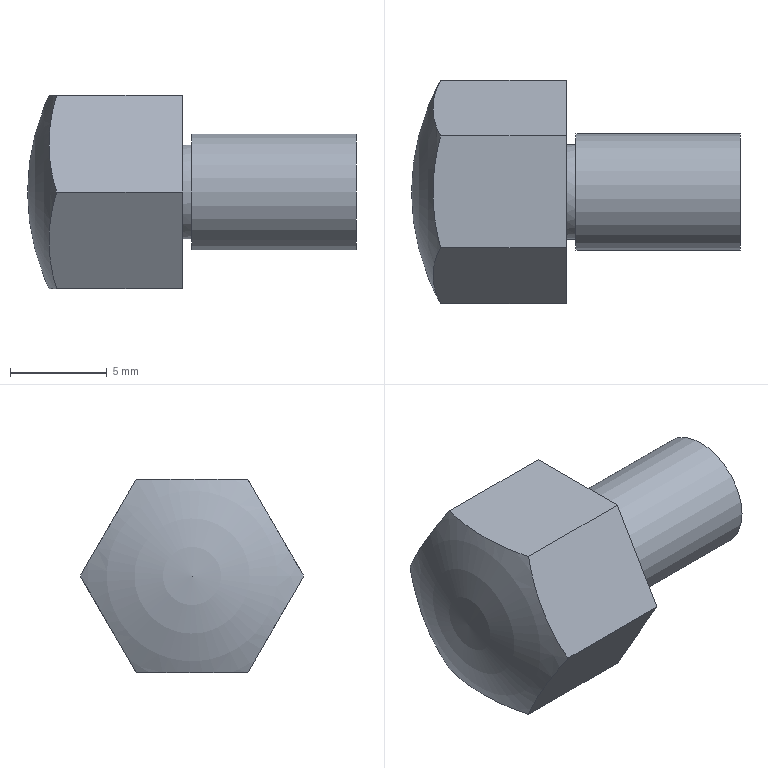Part | NX | features 5003_314_BSTEH10B 2 | 1 solid | 12 faces | box 17 x 11.547 x 10 mm | volume 889.716 mm3 | plane 9 | cylinder 2 | torus 1 | commonest cylinder face diameters 4.9 x1 6 x1
STEP:
#1=CARTESIAN_POINT('',(38.1,-177.774,-220.));
#2=VERTEX_POINT('',#1);
#3=CARTESIAN_POINT('',(38.1,-174.887,-215.));
#4=VERTEX_POINT('',#3);
#5=CARTESIAN_POINT('',(38.1,-177.774,-220.));
#6=CARTESIAN_POINT('',(37.578,-176.829,-218.364));
#7=CARTESIAN_POINT('',(37.578,-175.831,-216.636));
#8=CARTESIAN_POINT('',(38.1,-174.887,-215.));
#9=B_SPLINE_CURVE_WITH_KNOTS('',3,(#5,#6,#7,#8),.UNSPECIFIED.,.F.,.F.,(4,4),(0.000000237,0.00582),.UNSPECIFIED.);
#10=EDGE_CURVE('',#2,#4,#9,.T.);
#11=ORIENTED_EDGE('',*,*,#10,.F.);
#12=CARTESIAN_POINT('',(44.6,-177.774,-220.));
#13=VERTEX_POINT('',#12);
#14=CARTESIAN_POINT('',(36.6,-177.774,-220.));
#15=DIRECTION('',(1.,0.,0.));
#16=VECTOR('',#15,1000.);
#17=LINE('',#14,#16);
#18=EDGE_CURVE('',#2,#13,#17,.T.);
#19=ORIENTED_EDGE('',*,*,#18,.T.);
#20=CARTESIAN_POINT('',(44.6,-174.887,-215.));
#21=VERTEX_POINT('',#20);
#22=CARTESIAN_POINT('',(44.6,-174.887,-215.));
#23=DIRECTION('',(0.,-0.5,-0.866));
#24=VECTOR('',#23,1000.);
#25=LINE('',#22,#24);
#26=EDGE_CURVE('',#21,#13,#25,.T.);
#27=ORIENTED_EDGE('',*,*,#26,.F.);
#28=CARTESIAN_POINT('',(36.6,-174.887,-215.));
#29=DIRECTION('',(1.,0.,0.));
#30=VECTOR('',#29,1000.);
#31=LINE('',#28,#30);
#32=EDGE_CURVE('',#4,#21,#31,.T.);
#33=ORIENTED_EDGE('',*,*,#32,.F.);
#34=EDGE_LOOP('',(#11,#19,#27,#33));
#35=FACE_BOUND('',#34,.T.);
#36=CARTESIAN_POINT('',(36.6,-174.887,-215.));
#37=DIRECTION('',(0.,-0.866,0.5));
#38=DIRECTION('',(0.,-0.5,-0.866));
#39=AXIS2_PLACEMENT_3D('',#36,#37,#38);
#40=PLANE('',#39);
#41=ADVANCED_FACE('',(#35),#40,.T.);
#42=CARTESIAN_POINT('',(38.1,-169.113,-215.));
#43=VERTEX_POINT('',#42);
#44=CARTESIAN_POINT('',(38.1,-174.887,-215.));
#45=CARTESIAN_POINT('',(37.582,-173.011,-215.));
#46=CARTESIAN_POINT('',(37.582,-170.987,-215.));
#47=CARTESIAN_POINT('',(38.1,-169.113,-215.));
#48=B_SPLINE_CURVE_WITH_KNOTS('',3,(#44,#45,#46,#47),.UNSPECIFIED.,.F.,.F.,(4,4),(0.06513,0.07094),.UNSPECIFIED.);
#49=EDGE_CURVE('',#4,#43,#48,.T.);
#50=ORIENTED_EDGE('',*,*,#49,.F.);
#51=ORIENTED_EDGE('',*,*,#32,.T.);
#52=CARTESIAN_POINT('',(44.6,-169.113,-215.));
#53=VERTEX_POINT('',#52);
#54=CARTESIAN_POINT('',(44.6,-169.113,-215.));
#55=DIRECTION('',(0.,-1.,0.));
#56=VECTOR('',#55,1000.);
#57=LINE('',#54,#56);
#58=EDGE_CURVE('',#53,#21,#57,.T.);
#59=ORIENTED_EDGE('',*,*,#58,.F.);
#60=CARTESIAN_POINT('',(36.6,-169.113,-215.));
#61=DIRECTION('',(1.,0.,0.));
#62=VECTOR('',#61,1000.);
#63=LINE('',#60,#62);
#64=EDGE_CURVE('',#43,#53,#63,.T.);
#65=ORIENTED_EDGE('',*,*,#64,.F.);
#66=EDGE_LOOP('',(#50,#51,#59,#65));
#67=FACE_BOUND('',#66,.T.);
#68=CARTESIAN_POINT('',(36.6,-169.113,-215.));
#69=DIRECTION('',(0.,0.,1.));
#70=DIRECTION('',(-1.,0.,0.));
#71=AXIS2_PLACEMENT_3D('',#68,#69,#70);
#72=PLANE('',#71);
#73=ADVANCED_FACE('',(#67),#72,.T.);
#74=CARTESIAN_POINT('',(38.1,-166.226,-220.));
#75=VERTEX_POINT('',#74);
#76=CARTESIAN_POINT('',(38.1,-169.113,-215.));
#77=CARTESIAN_POINT('',(37.578,-168.169,-216.636));
#78=CARTESIAN_POINT('',(37.578,-167.171,-218.364));
#79=CARTESIAN_POINT('',(38.1,-166.226,-220.));
#80=B_SPLINE_CURVE_WITH_KNOTS('',3,(#76,#77,#78,#79),.UNSPECIFIED.,.F.,.F.,(4,4),(0.000000237,0.00582),.UNSPECIFIED.);
#81=EDGE_CURVE('',#43,#75,#80,.T.);
#82=ORIENTED_EDGE('',*,*,#81,.F.);
#83=ORIENTED_EDGE('',*,*,#64,.T.);
#84=CARTESIAN_POINT('',(44.6,-166.226,-220.));
#85=VERTEX_POINT('',#84);
#86=CARTESIAN_POINT('',(44.6,-166.226,-220.));
#87=DIRECTION('',(0.,-0.5,0.866));
#88=VECTOR('',#87,1000.);
#89=LINE('',#86,#88);
#90=EDGE_CURVE('',#85,#53,#89,.T.);
#91=ORIENTED_EDGE('',*,*,#90,.F.);
#92=CARTESIAN_POINT('',(36.6,-166.226,-220.));
#93=DIRECTION('',(1.,0.,0.));
#94=VECTOR('',#93,1000.);
#95=LINE('',#92,#94);
#96=EDGE_CURVE('',#75,#85,#95,.T.);
#97=ORIENTED_EDGE('',*,*,#96,.F.);
#98=EDGE_LOOP('',(#82,#83,#91,#97));
#99=FACE_BOUND('',#98,.T.);
#100=CARTESIAN_POINT('',(36.6,-166.226,-220.));
#101=DIRECTION('',(0.,0.866,0.5));
#102=DIRECTION('',(0.,-0.5,0.866));
#103=AXIS2_PLACEMENT_3D('',#100,#101,#102);
#104=PLANE('',#103);
#105=ADVANCED_FACE('',(#99),#104,.T.);
#106=CARTESIAN_POINT('',(38.1,-169.113,-225.));
#107=VERTEX_POINT('',#106);
#108=CARTESIAN_POINT('',(38.1,-166.226,-220.));
#109=CARTESIAN_POINT('',(37.578,-167.171,-221.636));
#110=CARTESIAN_POINT('',(37.578,-168.169,-223.364));
#111=CARTESIAN_POINT('',(38.1,-169.113,-225.));
#112=B_SPLINE_CURVE_WITH_KNOTS('',3,(#108,#109,#110,#111),.UNSPECIFIED.,.F.,.F.,(4,4),(0.000000237,0.00582),.UNSPECIFIED.);
#113=EDGE_CURVE('',#75,#107,#112,.T.);
#114=ORIENTED_EDGE('',*,*,#113,.F.);
#115=ORIENTED_EDGE('',*,*,#96,.T.);
#116=CARTESIAN_POINT('',(44.6,-169.113,-225.));
#117=VERTEX_POINT('',#116);
#118=CARTESIAN_POINT('',(44.6,-169.113,-225.));
#119=DIRECTION('',(0.,0.5,0.866));
#120=VECTOR('',#119,1000.);
#121=LINE('',#118,#120);
#122=EDGE_CURVE('',#117,#85,#121,.T.);
#123=ORIENTED_EDGE('',*,*,#122,.F.);
#124=CARTESIAN_POINT('',(36.6,-169.113,-225.));
#125=DIRECTION('',(1.,0.,0.));
#126=VECTOR('',#125,1000.);
#127=LINE('',#124,#126);
#128=EDGE_CURVE('',#107,#117,#127,.T.);
#129=ORIENTED_EDGE('',*,*,#128,.F.);
#130=EDGE_LOOP('',(#114,#115,#123,#129));
#131=FACE_BOUND('',#130,.T.);
#132=CARTESIAN_POINT('',(36.6,-169.113,-225.));
#133=DIRECTION('',(0.,0.866,-0.5));
#134=DIRECTION('',(0.,0.5,0.866));
#135=AXIS2_PLACEMENT_3D('',#132,#133,#134);
#136=PLANE('',#135);
#137=ADVANCED_FACE('',(#131),#136,.T.);
#138=CARTESIAN_POINT('',(38.1,-174.887,-225.));
#139=VERTEX_POINT('',#138);
#140=CARTESIAN_POINT('',(38.1,-169.113,-225.));
#141=CARTESIAN_POINT('',(37.582,-170.989,-225.));
#142=CARTESIAN_POINT('',(37.582,-173.013,-225.));
#143=CARTESIAN_POINT('',(38.1,-174.887,-225.));
#144=B_SPLINE_CURVE_WITH_KNOTS('',3,(#140,#141,#142,#143),.UNSPECIFIED.,.F.,.F.,(4,4),(0.06513,0.07094),.UNSPECIFIED.);
#145=EDGE_CURVE('',#107,#139,#144,.T.);
#146=ORIENTED_EDGE('',*,*,#145,.F.);
#147=ORIENTED_EDGE('',*,*,#128,.T.);
#148=CARTESIAN_POINT('',(44.6,-174.887,-225.));
#149=VERTEX_POINT('',#148);
#150=CARTESIAN_POINT('',(44.6,-174.887,-225.));
#151=DIRECTION('',(0.,1.,0.));
#152=VECTOR('',#151,1000.);
#153=LINE('',#150,#152);
#154=EDGE_CURVE('',#149,#117,#153,.T.);
#155=ORIENTED_EDGE('',*,*,#154,.F.);
#156=CARTESIAN_POINT('',(36.6,-174.887,-225.));
#157=DIRECTION('',(1.,0.,0.));
#158=VECTOR('',#157,1000.);
#159=LINE('',#156,#158);
#160=EDGE_CURVE('',#139,#149,#159,.T.);
#161=ORIENTED_EDGE('',*,*,#160,.F.);
#162=EDGE_LOOP('',(#146,#147,#155,#161));
#163=FACE_BOUND('',#162,.T.);
#164=CARTESIAN_POINT('',(36.6,-174.887,-225.));
#165=DIRECTION('',(0.,0.,-1.));
#166=DIRECTION('',(1.,0.,0.));
#167=AXIS2_PLACEMENT_3D('',#164,#165,#166);
#168=PLANE('',#167);
#169=ADVANCED_FACE('',(#163),#168,.T.);
#170=CARTESIAN_POINT('',(38.1,-174.887,-225.));
#171=CARTESIAN_POINT('',(37.578,-175.831,-223.364));
#172=CARTESIAN_POINT('',(37.578,-176.829,-221.636));
#173=CARTESIAN_POINT('',(38.1,-177.774,-220.));
#174=B_SPLINE_CURVE_WITH_KNOTS('',3,(#170,#171,#172,#173),.UNSPECIFIED.,.F.,.F.,(4,4),(0.000000237,0.00582),.UNSPECIFIED.);
#175=EDGE_CURVE('',#139,#2,#174,.T.);
#176=ORIENTED_EDGE('',*,*,#175,.F.);
#177=ORIENTED_EDGE('',*,*,#160,.T.);
#178=CARTESIAN_POINT('',(44.6,-177.774,-220.));
#179=DIRECTION('',(0.,0.5,-0.866));
#180=VECTOR('',#179,1000.);
#181=LINE('',#178,#180);
#182=EDGE_CURVE('',#13,#149,#181,.T.);
#183=ORIENTED_EDGE('',*,*,#182,.F.);
#184=ORIENTED_EDGE('',*,*,#18,.F.);
#185=EDGE_LOOP('',(#176,#177,#183,#184));
#186=FACE_BOUND('',#185,.T.);
#187=CARTESIAN_POINT('',(36.6,-177.774,-220.));
#188=DIRECTION('',(0.,-0.866,-0.5));
#189=DIRECTION('',(0.,0.5,-0.866));
#190=AXIS2_PLACEMENT_3D('',#187,#188,#189);
#191=PLANE('',#190);
#192=ADVANCED_FACE('',(#186),#191,.T.);
#193=CARTESIAN_POINT('',(44.6,-172.,-217.55));
#194=VERTEX_POINT('',#193);
#195=CARTESIAN_POINT('',(44.6,-172.,-220.));
#196=DIRECTION('',(1.,0.,0.));
#197=DIRECTION('',(0.,0.,1.));
#198=AXIS2_PLACEMENT_3D('',#195,#196,#197);
#199=CIRCLE('',#198,2.45);
#200=EDGE_CURVE('',#194,#194,#199,.T.);
#201=ORIENTED_EDGE('',*,*,#200,.F.);
#202=EDGE_LOOP('',(#201));
#203=FACE_BOUND('',#202,.T.);
#204=ORIENTED_EDGE('',*,*,#26,.T.);
#205=ORIENTED_EDGE('',*,*,#182,.T.);
#206=ORIENTED_EDGE('',*,*,#154,.T.);
#207=ORIENTED_EDGE('',*,*,#122,.T.);
#208=ORIENTED_EDGE('',*,*,#90,.T.);
#209=ORIENTED_EDGE('',*,*,#58,.T.);
#210=EDGE_LOOP('',(#204,#205,#206,#207,#208,#209));
#211=FACE_BOUND('',#210,.T.);
#212=CARTESIAN_POINT('',(44.6,-172.,-220.));
#213=DIRECTION('',(1.,0.,0.));
#214=DIRECTION('',(0.,0.,1.));
#215=AXIS2_PLACEMENT_3D('',#212,#213,#214);
#216=PLANE('',#215);
#217=ADVANCED_FACE('',(#203,#211),#216,.T.);
#218=ORIENTED_EDGE('',*,*,#200,.T.);
#219=EDGE_LOOP('',(#218));
#220=FACE_BOUND('',#219,.T.);
#221=CARTESIAN_POINT('',(45.1,-174.45,-220.));
#222=VERTEX_POINT('',#221);
#223=CARTESIAN_POINT('',(45.1,-172.,-220.));
#224=DIRECTION('',(1.,0.,0.));
#225=DIRECTION('',(0.,-1.,0.));
#226=AXIS2_PLACEMENT_3D('',#223,#224,#225);
#227=CIRCLE('',#226,2.45);
#228=EDGE_CURVE('',#222,#222,#227,.T.);
#229=ORIENTED_EDGE('',*,*,#228,.F.);
#230=EDGE_LOOP('',(#229));
#231=FACE_BOUND('',#230,.T.);
#232=CARTESIAN_POINT('',(53.6,-172.,-220.));
#233=DIRECTION('',(1.,0.,0.));
#234=DIRECTION('',(0.,-1.,0.));
#235=AXIS2_PLACEMENT_3D('',#232,#233,#234);
#236=CYLINDRICAL_SURFACE('',#235,2.45);
#237=ADVANCED_FACE('',(#220,#231),#236,.T.);
#238=ORIENTED_EDGE('',*,*,#228,.T.);
#239=EDGE_LOOP('',(#238));
#240=FACE_BOUND('',#239,.T.);
#241=CARTESIAN_POINT('',(45.1,-175.,-220.));
#242=VERTEX_POINT('',#241);
#243=CARTESIAN_POINT('',(45.1,-172.,-220.));
#244=DIRECTION('',(1.,0.,0.));
#245=DIRECTION('',(0.,-1.,0.));
#246=AXIS2_PLACEMENT_3D('',#243,#244,#245);
#247=CIRCLE('',#246,3.);
#248=EDGE_CURVE('',#242,#242,#247,.T.);
#249=ORIENTED_EDGE('',*,*,#248,.F.);
#250=EDGE_LOOP('',(#249));
#251=FACE_BOUND('',#250,.T.);
#252=CARTESIAN_POINT('',(45.1,-174.45,-220.));
#253=DIRECTION('',(-1.,0.,0.));
#254=DIRECTION('',(0.,1.,0.));
#255=AXIS2_PLACEMENT_3D('',#252,#253,#254);
#256=PLANE('',#255);
#257=ADVANCED_FACE('',(#240,#251),#256,.T.);
#258=ORIENTED_EDGE('',*,*,#248,.T.);
#259=EDGE_LOOP('',(#258));
#260=FACE_BOUND('',#259,.T.);
#261=CARTESIAN_POINT('',(53.6,-175.,-220.));
#262=VERTEX_POINT('',#261);
#263=CARTESIAN_POINT('',(53.6,-172.,-220.));
#264=DIRECTION('',(1.,0.,0.));
#265=DIRECTION('',(0.,-1.,0.));
#266=AXIS2_PLACEMENT_3D('',#263,#264,#265);
#267=CIRCLE('',#266,3.);
#268=EDGE_CURVE('',#262,#262,#267,.T.);
#269=ORIENTED_EDGE('',*,*,#268,.F.);
#270=EDGE_LOOP('',(#269));
#271=FACE_BOUND('',#270,.T.);
#272=CARTESIAN_POINT('',(53.6,-172.,-220.));
#273=DIRECTION('',(1.,0.,0.));
#274=DIRECTION('',(0.,-1.,0.));
#275=AXIS2_PLACEMENT_3D('',#272,#273,#274);
#276=CYLINDRICAL_SURFACE('',#275,3.);
#277=ADVANCED_FACE('',(#260,#271),#276,.T.);
#278=ORIENTED_EDGE('',*,*,#268,.T.);
#279=EDGE_LOOP('',(#278));
#280=FACE_BOUND('',#279,.T.);
#281=CARTESIAN_POINT('',(53.6,-175.,-220.));
#282=DIRECTION('',(1.,0.,0.));
#283=DIRECTION('',(0.,-1.,0.));
#284=AXIS2_PLACEMENT_3D('',#281,#282,#283);
#285=PLANE('',#284);
#286=ADVANCED_FACE('',(#280),#285,.T.);
#287=CARTESIAN_POINT('',(36.6,-172.,-220.));
#288=VERTEX_POINT('',#287);
#289=VERTEX_LOOP('',#288);
#290=FACE_BOUND('',#289,.T.);
#291=ORIENTED_EDGE('',*,*,#175,.T.);
#292=ORIENTED_EDGE('',*,*,#10,.T.);
#293=ORIENTED_EDGE('',*,*,#49,.T.);
#294=ORIENTED_EDGE('',*,*,#81,.T.);
#295=ORIENTED_EDGE('',*,*,#113,.T.);
#296=ORIENTED_EDGE('',*,*,#145,.T.);
#297=EDGE_LOOP('',(#291,#292,#293,#294,#295,#296));
#298=FACE_BOUND('',#297,.T.);
#299=CARTESIAN_POINT('',(48.6,-172.,-220.));
#300=DIRECTION('',(-1.,0.,0.));
#301=DIRECTION('',(0.,1.,0.));
#302=AXIS2_PLACEMENT_3D('',#299,#300,#301);
#303=DEGENERATE_TOROIDAL_SURFACE('',#302,0.03607,12.,.F.);
#304=ADVANCED_FACE('',(#290,#298),#303,.F.);
#305=CLOSED_SHELL('',(#41,#73,#105,#137,#169,#192,#217,#237,#257,#277,#286,#304));
#306=MANIFOLD_SOLID_BREP('',#305);
#307=(LENGTH_UNIT()NAMED_UNIT(*)SI_UNIT(.MILLI.,.METRE.));
#308=UNCERTAINTY_MEASURE_WITH_UNIT(LENGTH_MEASURE(0.0508),#307,'','');
#309=(NAMED_UNIT(*)PLANE_ANGLE_UNIT()SI_UNIT($,.RADIAN.));
#310=(NAMED_UNIT(*)SI_UNIT($,.STERADIAN.)SOLID_ANGLE_UNIT());
#311=(GEOMETRIC_REPRESENTATION_CONTEXT(3)GLOBAL_UNCERTAINTY_ASSIGNED_CONTEXT((#308))GLOBAL_UNIT_ASSIGNED_CONTEXT((#307,#309,#310))REPRESENTATION_CONTEXT('',''));
#312=ADVANCED_BREP_SHAPE_REPRESENTATION('',(#306),#311);